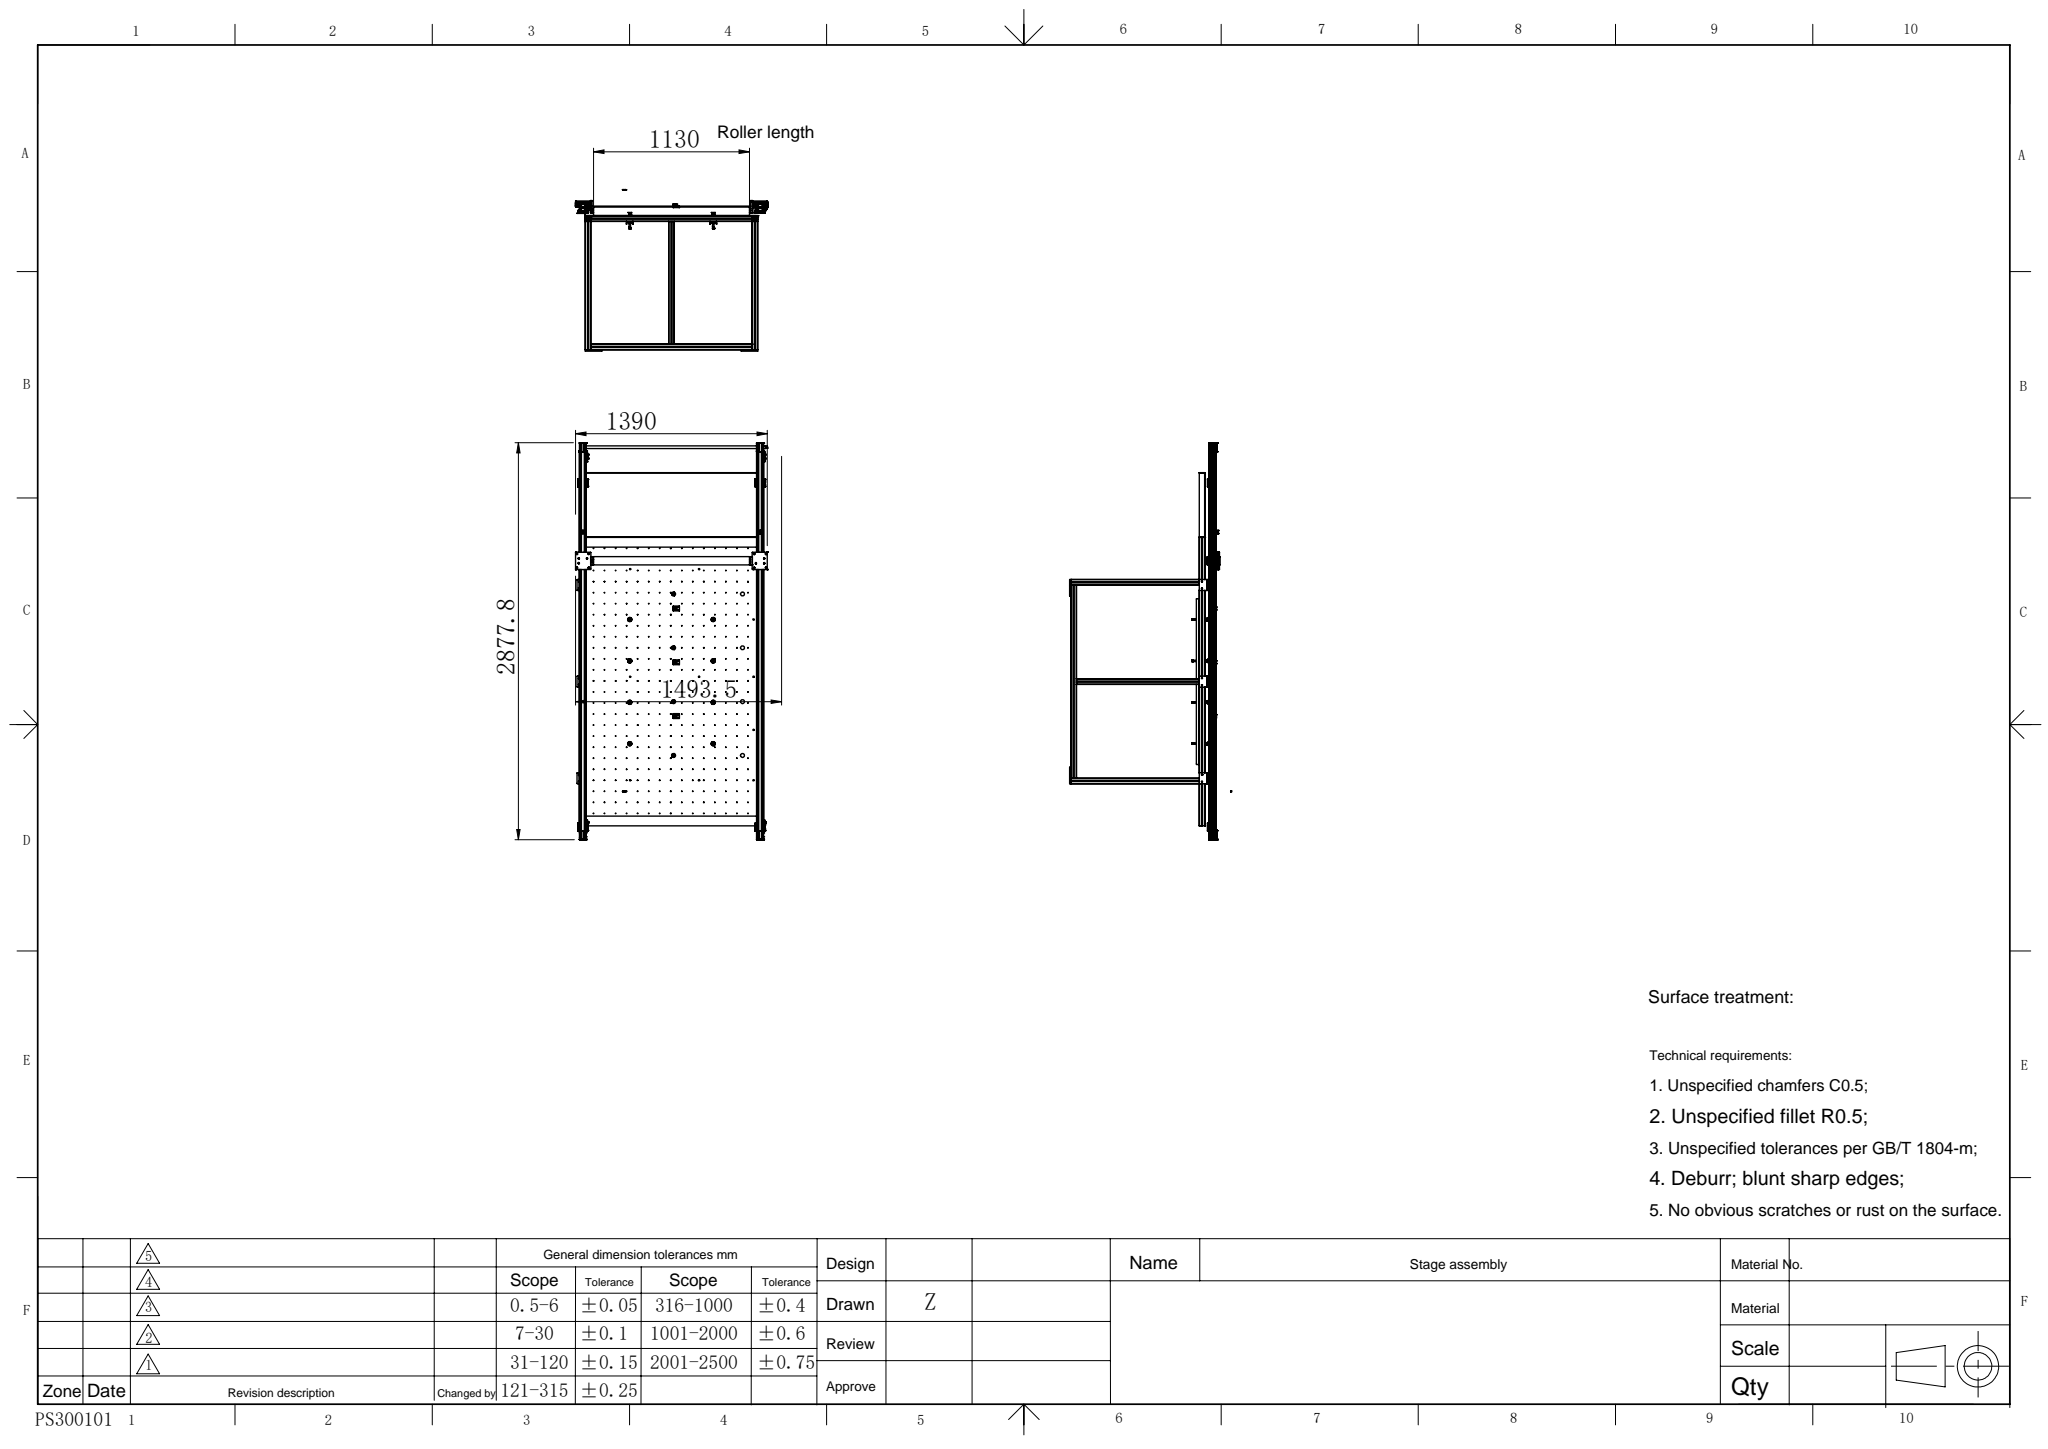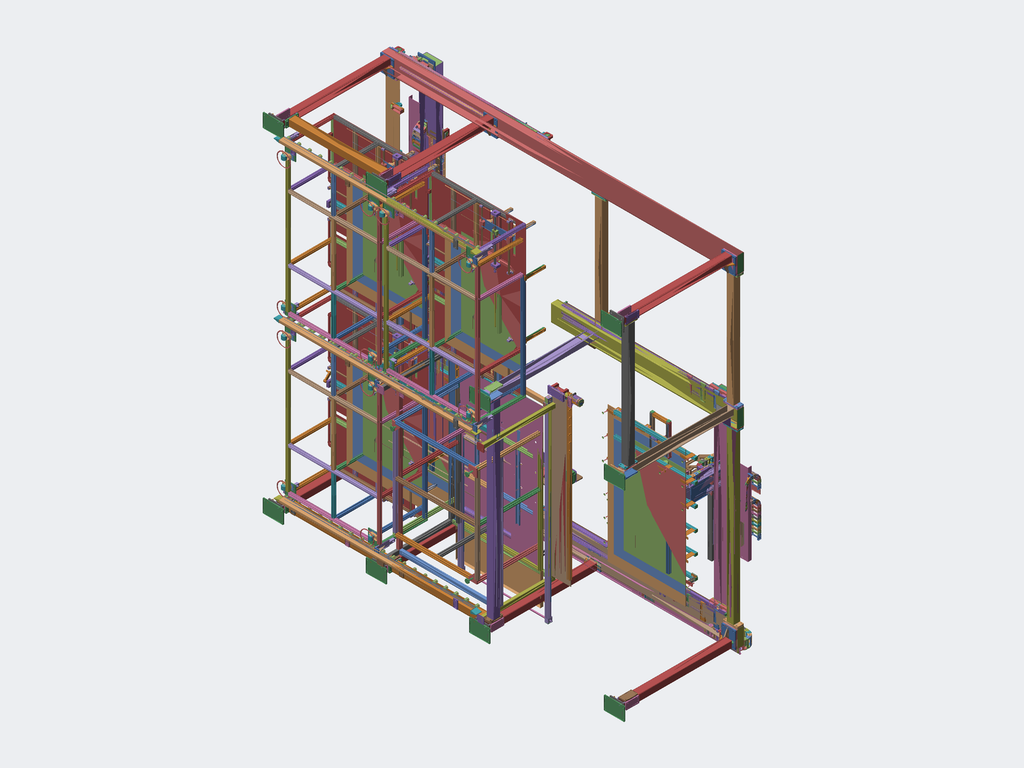Assembly | SolidWorks | 269 different items | 1682 placed
Parts list (item | name | quantity | parent item | size | volume | features):
1 | 57 Stepper and 400W Servo Reducer Pad | x1 | - | - | - | -
2 | (subassembly) | x1 | in 10 | - | - | features ReferencePattern 4, MirrorCompFeat 1
3 | (subassembly) | x1 | in 10 | - | - | features CompositeCurve 1
4 | (subassembly) | x1 | in 10 | - | - | features CompositeCurve 3
5 | (subassembly) | x1 | in 3 | - | - | features CompositeCurve 1, MirrorCompFeat 1, ReferencePattern 1
6 | (subassembly) | x1 | in 4 | - | - | features MirrorCompFeat 1, ReferencePattern 1
7 | (subassembly) | x1 | in 6 | - | 20673869 mm3 | features ReferencePattern 4, CompositeCurve 1, DerivedHolePattern 1
8 | (subassembly) | x1 | in 5 | - | 31071679 mm3 | features ReferencePattern 4, CompositeCurve 1, DerivedHolePattern 1
9 | (subassembly) | x2 | in 7, 8 | 105 x 90.9 x 98 mm | 242700 mm3 | -
10 | (subassembly) | x1 | - | - | - | features ReferencePattern 8, CompositeCurve 2, InContextFeatHolder 2, MirrorCompFeat 2
11 | (subassembly) | x3 | - | - | 40596234 mm3 | features ReferencePattern 157, MirrorCompFeat 6, LocalLPattern 1
12 | (subassembly) | x8 | in 20 | 34 x 24 x 440 mm | 99523 mm3 | -
13 | (subassembly) | x3 | in 3, 10, 15 | 234 x 112 x 120 mm | 1078897 mm3 | -
14 | (subassembly) | x1 | in 10 | 234 x 112 x 120 mm | 1078897 mm3 | -
15 | (subassembly) | x1 | - | - | 35795724 mm3 | features CompositeCurve 8, Belt 1, InContextFeatHolder 1
16 | (subassembly) | x8 | in 21 | 35 x 25 x 45.5 mm | 18401 mm3 | -
17 | (subassembly) | x24 | in 18, 19 | 63.895 x 210.5 x 120 mm | 48532 mm3 | features ReferencePattern 2, DerivedHolePattern 1
18 | (subassembly) | x6 | in 20 | - | 1484218 mm3 | features LocalLPattern 1, ReferencePattern 1
19 | (subassembly) | x6 | in 20 | - | 1567936 mm3 | features ReferencePattern 2, LocalLPattern 1, MirrorCompFeat 1
20 | (subassembly) | x2 | in 7, 8 | - | 15004104 mm3 | features ReferencePattern 15, CompositeCurve 4, MirrorCompFeat 4, LocalLPattern 1
21 | (subassembly) | x1 | in 39 | 2190 x 55.4 x 1350 mm | 56366306 mm3 | features ReferencePattern 7, DerivedHolePattern 1
22 | (subassembly) | x12 | in 18, 19 | 34 x 24 x 680 mm | 167801 mm3 | -
23 | (subassembly) | x2 | - | 2990 x 153 x 120 mm | 4241978 mm3 | features ReferencePattern 36, DerivedHolePattern 1
24 | (subassembly) | x1 | - | 2990 x 153 x 120 mm | 5333989 mm3 | features ReferencePattern 68, LocalLPattern 1
25 | (subassembly) | x1 | in 15 | 30 x 56 x 56 mm | 26536 mm3 | -
26 | (subassembly) | x6 | in 11 | 65 x 310 x 35 mm | 330251 mm3 | -
27 | (subassembly) | x18 | in 36, 37, 38 | 65 x 352 x 35 mm | 373958 mm3 | -
28 | (subassembly) | x3 | in 38 | 62 x 36.8 x 720 mm | 370830 mm3 | -
29 | (subassembly) | x1 | in 15 | 1250 x 163.16 x 142.786 mm | 4866204 mm3 | features CompositeCurve 1
30 | (subassembly) | x2 | in 10 | 250 x 77 x 220 mm | 2116355 mm3 | -
31 | (subassembly) | x1 | in 3 | 250 x 77 x 220 mm | 1248427 mm3 | -
32 | (subassembly) | x2 | in 7, 8 | 30 x 45 x 61.9 mm | 25881 mm3 | -
33 | (subassembly) | x4 | in 10 | 60 x 45 x 2040 mm | 1527513 mm3 | -
34 | (subassembly) | x4 | in 3, 10, 15 | 230 x 112 x 120 mm | 1042878 mm3 | -
35 | (subassembly) | x1 | - | 31 x 72 x 130 mm | 56690 mm3 | -
36 | (subassembly) | x3 | in 11 | 465.166 x 413.18 x 727.5 mm | 2675424 mm3 | -
37 | (subassembly) | x3 | in 11 | 465 x 411 x 721.167 mm | 2675425 mm3 | -
38 | (subassembly) | x3 | in 11 | 866.479 x 413.5 x 727.5 mm | 3012478 mm3 | features MirrorCompFeat 1, ReferencePattern 1
39 | (subassembly) | x1 | - | - | 36230878 mm3 | features ReferencePattern 5, InContextFeatHolder 2, LocalLPattern 1, MirrorCompFeat 1
40 | (subassembly) | x2 | in 7, 8 | 152.95 x 49 x 57.5 mm | 133914 mm3 | features ReferencePattern 5, DerivedHolePattern 1
41 | (subassembly) | x12 | in 18, 19 | 109 x 59.2 x 29.612 mm | 63942 mm3 | features ReferencePattern 7, DerivedHolePattern 1, MirrorCompFeat 1
42 | (subassembly) | x1 | in 39 | - | 15688667 mm3 | features CompositeCurve 1, MirrorCompFeat 1, ReferencePattern 1
43 | (subassembly) | x2 | in 39 | 1200 x 50 x 118 mm | 235695 mm3 | features ReferencePattern 3, LocalLPattern 1
44 | (subassembly) | x3 | in 3 | 60 x 45 x 2850 mm | 1999576 mm3 | -
45 | (subassembly) | x2 | in 46 | - | 2196396 mm3 | features CompositeCurve 3
46 | (subassembly) | x2 | in 42 | - | 6127819 mm3 | features CompositeCurve 10
47 | (subassembly) | x1 | in 4 | 60 x 45 x 920 mm | 875210 mm3 | -
48 | (subassembly) | x2 | in 10 | - | 18345669 mm3 | -
49 | (subassembly) | x8 | in 13, 14, 34 | 89 x 61 x 61 mm | 120828 mm3 | -
50 | (subassembly) | x36 | in 36, 37, 38 | 60 x 55 x 35 mm | 37476 mm3 | -
51 | - | x12 | in 11 | 204.978 x 96 x 204.978 mm | 270055 mm3 | features BaseBody 4, BossThin 1
52 | - | x16 | in 20 | 65 x 34 x 40 mm | 63388 mm3 | features Chamfer 2, HoleWzd 2, Extrusion 1, ICE 1
53 | - | x2 | in 40 | 130 x 30 x 30 mm | 99886 mm3 | features HoleWzd 3, Chamfer 1, Extrusion 1
54 | - | x12 | in 41 | 90 x 30 x 18 mm | 41486 mm3 | features HoleWzd 3, Chamfer 1, Extrusion 1
55 | - | x12 | in 11 | 40 x 30 x 200 mm | 236731 mm3 | features Extrusion 1, HoleWzd 1
56 | - | x26 | in 18, 19, 20 | 40 x 12 x 20 mm | 5424 mm3 | features Chamfer 1, Extrusion 1, HoleWzd 1, ICE 1
57 | - | x4 | in 20 | 46 x 52 x 50 mm | 46820 mm3 | features HoleWzd 2, ICE 2, Chamfer 1, Extrusion 1
58 | - | x4 | in 20 | 430 x 10 x 30 mm | 124086 mm3 | features HoleWzd 2, Chamfer 1, Extrusion 1
59 | - | x2 | in 7, 8 | 230 x 12 x 330 mm | 777440 mm3 | features HoleWzd 3, Chamfer 1, Extrusion 1, Fillet 1, ICE 1
60 | - | x12 | in 18, 19 | 680 x 10 x 47.5 mm | 316323 mm3 | features HoleWzd 2, Chamfer 1, Extrusion 1
61 | - | x2 | in 20 | 380 x 15 x 270 mm | 1473539 mm3 | features ICE 4, HoleWzd 2, Chamfer 1, Extrusion 1
62 | - | x6 | in 11 | 31 x 50 x 50 mm | 48468 mm3 | features BaseBody 1
63 | - | x2 | in 7 | 220 x 12 x 735 mm | 1211217 mm3 | features HoleWzd 8, ICE 2, Chamfer 1, Extrusion 1, Fillet 1
64 | - | x10 | in 7, 8 | 15 x 168 x 15 mm | 28790 mm3 | features Chamfer 1, Extrusion 1, HoleWzd 1, ICE 1, MirrorPattern 1
65 | - | x1 | in 7 | 192 x 15 x 200 mm | 382699 mm3 | features HoleWzd 2, Chamfer 1, Extrusion 1, ICE 1
66 | - | x2 | in 8 | 220 x 12 x 802 mm | 1372017 mm3 | features HoleWzd 8, ICE 2, Chamfer 1, Extrusion 1, Fillet 1
67 | - | x6 | in 11 | 13 x 44.5 x 11 mm | 2225 mm3 | features ICE 3, Chamfer 1, Extrusion 1, RevCut 1
68 | - | x1 | - | 30 x 10 x 126 mm | 36512 mm3 | features HoleWzd 2, Chamfer 1, Extrusion 1
69 | - | x8 | in 16 | 45 x 18.5 x 35 mm | 16639 mm3 | features HoleWzd 2, ICE 2, Chamfer 1, Extrusion 1
70 | - | x4 | - | 60 x 210 x 80 mm | 235958 mm3 | features ICE 3, Chamfer 2, Extrusion 1
71 | - | x3 | in 39 | 60 x 179 x 60 mm | 83421 mm3 | features BaseBody 2
72 | - | x16 | in 13, 14, 34 | 25 x 95 x 100 mm | 157637 mm3 | features HoleWzd 3, ICE 3, Chamfer 2, Extrusion 1
73 | - | x4 | in 13, 14 | 230 x 20 x 100 mm | 414284 mm3 | features HoleWzd 4, Chamfer 1, Extrusion 1, ICE 1
74 | - | x4 | in 13, 14 | 204 x 36 x 36 mm | 132992 mm3 | features ICE 2, Chamfer 1, Revolution 1
75 | - | x16 | in 13, 14, 34 | 18.5 x 40 x 40 mm | 10029 mm3 | features Chamfer 1, Extrusion 1
76 | - | x16 | in 13, 14, 34 | 20 x 25 x 25 mm | 7188 mm3 | features Extrusion 1, HoleWzd 1
77 | - | x4 | in 34 | 169 x 40 x 40 mm | 119602 mm3 | features Chamfer 1, ICE 1, Revolution 1
78 | - | x5 | in 30, 31 | 250 x 77 x 65 mm | 889815 mm3 | features HoleWzd 6, ICE 2, Chamfer 1, Extrusion 1, MirrorPattern 1
79 | - | x6 | in 30, 31 | 70 x 10 x 190 mm | 129097 mm3 | features HoleWzd 2, Chamfer 1, Extrusion 1
80 | - | x2 | in 10 | 20 x 20 x 2135 mm | 670495 mm3 | features Chamfer 1, Extrusion 1
81 | - | x1 | in 10 | 160 x 15 x 160 mm | 370289 mm3 | features HoleWzd 2, Chamfer 1, Extrusion 1
82 | - | x4 | in 3, 10, 15 | 55 x 55 x 57 mm | 102625 mm3 | features BaseBody 1
83 | - | x2 | in 3, 15 | 120 x 117 x 50 mm | 147908 mm3 | features ICE 3, Chamfer 2, HoleWzd 2, Extrusion 1, MirrorSolid 1
84 | - | x4 | in 34 | 230 x 20 x 100 mm | 391656 mm3 | features HoleWzd 3, Chamfer 1, Extrusion 1, ICE 1
85 | - | x3 | in 11 | - | 21852981 mm3 | features WeldCornerFeat 2, 3DProfileFeature 1, WeldMemberFeat 1, WeldmentFeature 1
86 | - | x12 | in 18, 19 | 1200 x 40 x 40 mm | 725812 mm3 | features WeldMemberFeat 1, WeldmentFeature 1
87 | - | x1 | in 39 | 1250 x 970 x 2090 mm | 12416282 mm3 | features ICE 8, Extrusion 1
88 | - | x2 | in 20 | 1940 x 40 x 280 mm | 2830666 mm3 | features WeldMemberFeat 1, WeldmentFeature 1
89 | - | x1 | in 3 | 5030 x 162 x 315 mm | 22440671 mm3 | features ICE 11, HoleWzd 10, Chamfer 1, MirrorSolid 1, WeldMemberFeat 1, WeldmentFeature 1
90 | - | x1 | in 39 | 1590 x 1030 x 1350 mm | 17668090 mm3 | features HoleWzd 4, ICE 3, 3DProfileFeature 1, WeldCornerFeat 1, WeldMemberFeat 1, WeldmentFeature 1
91 | - | x1 | in 10 | 2745 x 1798 x 315 mm | 19263192 mm3 | features ICE 8, HoleWzd 5, MirrorSolid 4, WeldMemberFeat 2, LPattern 1, WeldCornerFeat 1, WeldmentFeature 1
92 | - | x1 | in 4 | 2945 x 142 x 275 mm | 8968186 mm3 | features HoleWzd 7, ICE 5, MirrorSolid 3, Chamfer 2, WeldMemberFeat 1, WeldmentFeature 1
93 | - | x2 | in 10 | - | - | features RefSurface 2
94 | - | x1 | in 10 | 2525 x 210 x 100 mm | 3620734 mm3 | features ICE 3, HoleWzd 2, WeldMemberFeat 2, LPattern 1, MirrorSolid 1, WeldCornerFeat 1, WeldmentFeature 1
95 | - | x1 | in 10 | 4500 x 230 x 153.7 mm | 8314769 mm3 | features ICE 5, HoleWzd 3, MirrorSolid 2, WeldMemberFeat 2, LPattern 1, WeldCornerFeat 1, WeldmentFeature 1
96 | - | x3 | in 23, 24 | 2990 x 95 x 120 mm | 3021491 mm3 | features ICE 5, MirrorSolid 2, HoleWzd 1, WeldMemberFeat 1, WeldmentFeature 1
97 | - | x1 | in 10 | 5240 x 145 x 265 mm | 27147429 mm3 | features ICE 9, HoleWzd 7, DeleteBody 1, MirrorSolid 1, WeldCornerFeat 1, WeldMemberFeat 1, WeldmentFeature 1
98 | - | x1 | in 10 | 5240 x 145 x 265 mm | 23826914 mm3 | features ICE 7, HoleWzd 6, Cut 1, DeleteBody 1, LPattern 1, MirrorSolid 1, WeldCornerFeat 1, WeldMemberFeat 1, WeldmentFeature 1
99 | - | x7 | in 10 | 200 x 1668 x 300 mm | 4715517 mm3 | features ICE 6, HoleWzd 4, CirPattern 2, DeleteBody 1, MirrorSolid 1, RefAxis 1, WeldCornerFeat 1, WeldMemberFeat 1, WeldmentFeature 1
100 | - | x3 | in 10 | 1395 x 100 x 190 mm | 2190418 mm3 | features HoleWzd 1, ICE 1, MirrorSolid 1, WeldMemberFeat 1, WeldmentFeature 1
101 | - | x1 | in 10 | 2825 x 100 x 190 mm | 3924535 mm3 | features HoleWzd 1, ICE 1, MirrorSolid 1, WeldMemberFeat 1, WeldmentFeature 1
102 | - | x1 | in 10 | 1845 x 100 x 190 mm | 2736119 mm3 | features HoleWzd 1, ICE 1, MirrorSolid 1, WeldMemberFeat 1, WeldmentFeature 1
103 | - | x2 | in 10 | 1695 x 100 x 210 mm | 2614218 mm3 | features HoleWzd 1, ICE 1, MirrorSolid 1, WeldMemberFeat 1, WeldmentFeature 1
104 | - | x6 | in 11 | 59 x 25 x 25 mm | 17907 mm3 | features BaseBody 4
105 | - | x1 | in 39 | 2090 x 2.5 x 1250 mm | 5366829 mm3 | features HoleWzd 3, ICE 3, Fillet 2, Extrusion 1
106 | - | x1 | in 15 | 1748 x 110 x 139.4 mm | 4195006 mm3 | features Fillet 2, ICE 2, Extrusion 1
107 | - | x28 | in 17, 20 | 15 x 46 x 15 mm | 3087 mm3 | features BaseBody 1
108 | - | x8 | in 16 | 26 x 10.5 x 26 mm | 1762 mm3 | features BaseBody 2
109 | - | x2 | in 32 | 30 x 45 x 61.9 mm | 24324 mm3 | features BaseBody 3
110 | - | x1 | in 15 | 1374 x 89 x 40 mm | 612800 mm3 | features Extrusion 1, ICE 1, MirrorPattern 1
111 | - | x1 | in 29 | 1200 x 10 x 80 mm | 959446 mm3 | features Extrusion 1, ICE 1
112 | - | x2 | in 15 | 86 x 60.5 x 139.4 mm | 512577 mm3 | features BaseBody 1
113 | - | x2 | in 15 | 45 x 38 x 2380 mm | 3190099 mm3 | features ICE 3, LPattern 2, BaseBody 1, RevCut 1
114 | - | x2 | in 15 | 86 x 25 x 53.5 mm | 94926 mm3 | features ICE 15, Chamfer 1, Extrusion 1, MirrorPattern 1, RevCut 1, Revolution 1
115 | - | x6 | in 3, 10 | 13.6 x 15.5 x 27.7 mm | 2033 mm3 | features BaseBody 1
116 | - | x74 | in 23, 24 | 68 x 13 x 13 mm | 3917 mm3 | features BaseBody 1
117 | - | x1 | in 3 | 80 x 59.15 x 3062 mm | 2509466 mm3 | features BossThin 1, ExtruThin 1
118 | - | x6 | in 30, 31 | 105 x 8 x 57 mm | 39266 mm3 | features HoleWzd 1, WeldMemberFeat 1, WeldmentFeature 1
119 | - | x8 | in 48 | 15.82 x 15.82 x 12 mm | 1643 mm3 | features BaseBody 1
120 | - | x8 | in 48 | 34 x 19.5 x 56.8 mm | 30476 mm3 | features BaseBody 1
121 | - | x2 | in 48 | 20 x 70 x 12 mm | 2355 mm3 | features BaseBody 1
122 | - | x6 | in 48 | 27 x 19 x 20 mm | 1847 mm3 | features BaseBody 1
123 | - | x2 | in 48 | 1.5 x 54 x 30 mm | 1466 mm3 | features BaseBody 1
124 | - | x6 | in 48 | 27.5 x 14 x 16 mm | 2237 mm3 | features BaseBody 1
125 | - | x2 | in 48 | 175 x 66 x 2404 mm | 15856732 mm3 | features BaseBody 3
126 | - | x8 | in 12 | 15 x 12.5 x 440 mm | 69027 mm3 | features ICE 2, BaseBody 1, HoleWzd 1
127 | - | x2 | in 48 | 270 x 54 x 195 mm | 1409975 mm3 | features BaseBody 1
128 | - | x2 | in 48 | 58.084 x 15.975 x 10 mm | 3195 mm3 | features BaseBody 3
129 | - | x4 | in 48 | 32 x 93.5 x 175 mm | 238017 mm3 | features BaseBody 1
130 | - | x4 | in 48 | 8 x 31 x 160 mm | 21339 mm3 | features BaseBody 1
131 | - | x4 | in 48 | 12 x 16 x 130 mm | 19917 mm3 | features BaseBody 1
132 | - | x2 | in 48 | 2454 x 50 x 130 mm | 330700 mm3 | features BaseBody 1
133 | - | x2 | in 48 | 64 x 15 x 7.5 mm | 6074 mm3 | features BaseBody 1
134 | - | x2 | in 48 | 1.5 x 10 x 2344 mm | 35160 mm3 | features BaseBody 1
135 | - | x2 | in 15 | 150 x 16 x 16 mm | 30147 mm3 | features ICE 7, RevCut 2, Chamfer 1, Revolution 1
136 | - | x9 | in 28, 36, 37 | 25 x 25 x 720 mm | 328967 mm3 | features ICE 5, Chamfer 2, Extrusion 1
137 | - | x12 | in 22 | 15 x 12.5 x 680 mm | 106806 mm3 | features ICE 2, BaseBody 1, HoleWzd 1
138 | - | x1 | in 29 | 60 x 60 x 1250 mm | 3405863 mm3 | features ICE 2, Extrusion 1, MirrorPattern 1
139 | - | x1 | in 29 | 1250 x 145.623 x 130.346 mm | 500895 mm3 | features ICE 5, Fillet 2, Extrusion 1, LPattern 1, Sweep 1
140 | - | x2 | in 10 | 80 x 59.15 x 2252 mm | 1851098 mm3 | features BossThin 1, ExtruThin 1
141 | - | x2 | in 15 | 50 x 38.5 x 23.5 mm | 34722 mm3 | features Extrusion 1, ICE 1
142 | - | x12 | in 19 | 20 x 20 x 15 mm | 3713 mm3 | features Extrusion 1, HoleWzd 1
143 | - | x4 | in 3, 10 | 6 x 9 x 250 mm | 7894 mm3 | features Extrusion 1, HoleWzd 1
144 | - | x18 | in 36, 37, 38 | 20 x 20 x 690 mm | 216754 mm3 | features Chamfer 1, Extrusion 1
145 | - | x1 | in 15 | 1794 x 1094 x 2450 mm | 14966587 mm3 | features ICE 8, Extrusion 1
146 | - | x1 | in 42 | 92 x 60 x 12 mm | 51329 mm3 | features MirrorStock 1
147 | - | x1 | in 39 | 1250 x 470 x 42 mm | 1441666 mm3 | features EdgeFlange 1, FlatPattern 1, ICE 1, LPattern 1, SMBaseFlange 1, SheetMetal 1
148 | - | x32 | in 12, 22 | 34 x 19.5 x 57.8 mm | 30496 mm3 | features BaseBody 1
149 | - | x6 | in 39 | 80 x 60 x 60 mm | 27475 mm3 | features HoleWzd 2, EdgeFlange 1, Fillet 1, FlatPattern 1, SMBaseFlange 1, SheetMetal 1
150 | - | x2 | in 43 | 1200 x 50 x 20 mm | 201265 mm3 | features EdgeFlange 1, Fillet 1, FlatPattern 1, HoleWzd 1, ICE 1, SMBaseFlange 1, SheetMetal 1
151 | - | x2 | in 42 | 126 x 110 x 10 mm | 134120 mm3 | features HoleWzd 2, Chamfer 1, Extrusion 1
152 | - | x1 | in 42 | 92 x 60 x 12 mm | 51329 mm3 | features HoleWzd 2, ICE 2, Chamfer 1, Extrusion 1, Fillet 1
153 | - | x1 | in 42 | 60 x 60 x 1176 mm | 3172741 mm3 | features HoleWzd 2, ICE 2, Extrusion 1
154 | - | x1 | in 42 | 20 x 20 x 1300 mm | 408407 mm3 | features Extrusion 1
155 | - | x2 | in 46 | 39 x 39 x 49 mm | 38785 mm3 | features ICE 15, RevCut 7, CirPattern 3, Emboss 2, MirrorPattern 1, Revolution 1
156 | - | x2 | in 45 | 105 x 79 x 220 mm | 575496 mm3 | features BaseBody 33
157 | - | x6 | in 46 | 79.5 x 156 x 47 mm | 158160 mm3 | features BaseBody 3, MoveFace 2, ICE 1
158 | - | x2 | in 46 | 79.5 x 156 x 47 mm | 157908 mm3 | features BaseBody 3, MoveFace 2, ICE 1
159 | - | x32 | in 18, 19, 20 | 40 x 5 x 40 mm | 7913 mm3 | features Extrusion 1, Fillet 1
160 | - | x58 | in 17, 18, 19, 20, 43 | 28 x 118 x 28 mm | 8607 mm3 | features BaseBody 3
161 | - | x2 | in 46 | 87.3 x 177.09 x 47 mm | 222121 mm3 | features MoveFace 4, BaseBody 3, ICE 2
162 | - | x2 | in 46 | 87.3 x 177.09 x 47 mm | 215586 mm3 | features BaseBody 3, MoveFace 3, ICE 2
163 | - | x4 | in 46 | 105 x 52 x 165 mm | 515156 mm3 | features BaseBody 3
164 | - | x2 | in 46 | 105 x 52 x 220 mm | 691685 mm3 | features BaseBody 3
165 | - | x2 | in 46 | 105 x 52 x 126 mm | 392725 mm3 | features BaseBody 4
166 | - | x4 | in 46 | 60 x 60 x 112 mm | 219786 mm3 | features BaseBody 3
167 | - | x4 | in 46 | - | - | features RefSurface 50
168 | - | x2 | in 46 | 35 x 44 x 44 mm | 38152 mm3 | features BaseBody 10
169 | - | x2 | in 46 | - | - | features RefSurface 12
170 | - | x8 | in 46 | 59.5 x 59.5 x 14.7 mm | 28959 mm3 | features HoleWzd 3, ICE 3, CirPattern 2, Fillet 2, Chamfer 1, Cut 1, Extrusion 1, MirrorPattern 1
171 | - | x1 | in 7 | 135 x 141 x 169.1 mm | 931698 mm3 | features BaseBody 2
172 | - | x2 | in 46 | 106 x 62 x 74 mm | 204451 mm3 | features BaseBody 13, ICE 5, Chamfer 3
173 | - | x2 | in 46 | 86 x 62 x 74 mm | 199634 mm3 | features BaseBody 13, ICE 6, Chamfer 3
174 | - | x4 | in 46 | 59.5 x 62 x 74 mm | 191803 mm3 | features BaseBody 13, ICE 4, Chamfer 2
175 | - | x2 | in 46 | 79.5 x 62 x 74 mm | 200359 mm3 | features BaseBody 13, ICE 3, Chamfer 2
176 | - | x2 | in 46 | 106 x 62 x 74 mm | 204451 mm3 | features BaseBody 13, ICE 5, Chamfer 3, DeleteBody 1, MirrorSolid 1
177 | - | x2 | in 46 | 86 x 62 x 74 mm | 199635 mm3 | features BaseBody 13, ICE 6, Chamfer 3, DeleteBody 1, MirrorSolid 1
178 | - | x2 | in 46 | 59.5 x 62 x 74 mm | 191804 mm3 | features BaseBody 13, ICE 4, Chamfer 2, DeleteBody 1, MirrorSolid 1
179 | - | x2 | in 46 | 79.5 x 62 x 74 mm | 200359 mm3 | features BaseBody 13, ICE 3, Chamfer 2, DeleteBody 1, MirrorSolid 1
180 | - | x4 | in 46 | 60.5 x 118.5 x 60.5 mm | 241824 mm3 | features MBimport 1
181 | - | x4 | in 46 | - | - | features RefSurface 11
182 | - | x1 | in 35 | 31 x 72 x 130 mm | 55783 mm3 | features BaseBody 1
183 | - | x16 | in 33, 44, 47 | 60 x 39.001 x 97.7 mm | 170718 mm3 | features BaseBody 1
184 | - | x1 | in 47 | 28 x 26 x 920 mm | 533776 mm3 | features ICE 2, BaseBody 1, HoleWzd 1
185 | - | x3 | in 44 | 28 x 26 x 2850 mm | 1658147 mm3 | features ICE 2, BaseBody 1, HoleWzd 1
186 | - | x4 | in 33 | 28 x 26 x 2040 mm | 1186082 mm3 | features BaseBody 1, HoleWzd 1, ICE 1
187 | - | x1 | in 10 | 40.704 x 156.673 x 40.704 mm | 14106 mm3 | features BaseBody 2
188 | - | x1 | in 10 | 224 x 110 x 250 mm | 1662624 mm3 | features BaseBody 14
189 | - | x9 | in 28, 36, 37 | 36.8 x 62 x 50 mm | 41876 mm3 | features BaseBody 1
190 | - | x3 | in 39 | 120 x 120 x 10 mm | 110461 mm3 | features Extrusion 1, HoleWzd 1
191 | - | x18 | in 36, 37, 38 | 54 x 41 x 96 mm | 148221 mm3 | features BaseBody 1
192 | - | x4 | in 3, 4, 10, 15 | - | - | features RefSurface 26, BaseBody 15
193 | - | x2 | in 5, 6 | - | - | features RefSurface 26, BaseBody 20
194 | - | x1 | in 7 | - | - | features RefSurface 65
195 | - | x1 | in 10 | 110 x 224 x 250 mm | 2228860 mm3 | features BaseBody 34
196 | - | x1 | in 7 | - | - | features BaseBody 60, RefSurface 7
197 | - | x10 | in 3, 10, 31 | 13 x 15.011 x 68 mm | 5094 mm3 | features BaseBody 1
198 | - | x10 | in 3, 10, 31 | 12 x 18 x 38 mm | 5849 mm3 | features BaseBody 1
199 | - | x2 | in 40 | 39.583 x 28.95 x 18 mm | 7377 mm3 | features BaseBody 1
200 | - | x2 | in 32 | 24.119 x 17 x 10.238 mm | 1557 mm3 | features BaseBody 1
201 | - | x6 | in 11, 20, 21 | 2010 x 50 x 1150 mm | 11975475 mm3 | features ICE 5, Extrusion 1
202 | - | x120 | in 17, 41 | 28.619 x 17.5 x 12.5 mm | 2253 mm3 | features BaseBody 1
203 | - | x24 | in 40, 41 | 33.351 x 25 x 15 mm | 4442 mm3 | features BaseBody 1
204 | - | x2 | in 5, 6 | 384.7 x 122 x 879.7 mm | 13861724 mm3 | features BaseBody 11
205 | - | x1 | in 4 | 1047 x 122 x 230 mm | 15190033 mm3 | features BaseBody 6, LPattern 1
206 | - | x16 | in 49 | 61 x 61 x 2.5 mm | 4721 mm3 | features ICE 2, BaseBody 1
207 | - | x8 | in 49 | 84 x 54.65 x 54.249 mm | 111386 mm3 | features CirPattern 1, Cut 1, HoleWzd 1, ICE 1, WeldMemberFeat 1, WeldmentFeature 1
208 | - | x36 | in 50 | 60 x 51 x 20 mm | 29381 mm3 | features BaseBody 1
209 | - | x8 | in 19, 20 | 94 x 36 x 36 mm | 78823 mm3 | features BaseBody 2
210 | - | x1 | in 5 | 13 x 13 x 17.5 mm | 922.307 mm3 | features BaseBody 1
211 | - | x1 | in 3 | 90 x 90.211 x 179.85 mm | 785388 mm3 | features BaseBody 7
212 | - | x1 | in 3 | 90.02 x 90.185 x 188 mm | 989855 mm3 | features BaseBody 2
213 | - | x6 | in 10 | 127 x 65 x 37 mm | 109868 mm3 | features BaseBody 1
214 | - | x1 | in 4 | - | 2054187 mm3 | features BaseBody 18, LPattern 4
215 | - | x3 | in 2, 3 | - | - | features BaseBody 38, LPattern 5
216 | - | x2 | in 5, 6 | - | 1173984 mm3 | features BaseBody 14, LPattern 4
217 | - | x6 | in 11 | 630 x 56 x 28 mm | 285971 mm3 | features BaseBody 1
218 | - | x3 | in 11 | 2220 x 2 x 1390 mm | 5915480 mm3 | features Fillet 2, ICE 2, FlatPattern 1, HoleWzd 1, SMBaseFlange 1, SheetMetal 1
219 | - | x2 | in 5, 6 | 102 x 570 x 30 mm | 144671 mm3 | features HoleWzd 3, Fillet 1, FlatPattern 1, SMBaseFlange 1, SheetMetal 1
220 | - | x2 | in 6, 8 | 115 x 30 x 60 mm | 24246 mm3 | features HoleWzd 3, Fillet 1, FlatPattern 1, SMBaseFlange 1, SheetMetal 1
221 | - | x1 | in 3 | 202 x 70 x 3780 mm | 2020331 mm3 | features HoleWzd 3, Fillet 1, FlatPattern 1, ICE 1, SMBaseFlange 1, SheetMetal 1
222 | - | x2 | in 5, 6 | 225 x 23 x 70 mm | 48684 mm3 | features HoleWzd 3, Fillet 1, FlatPattern 1, ICE 1, Jog 1, SMBaseFlange 1, SheetMetal 1
223 | - | x18 | in 36, 37, 38 | 12 x 42 x 42 mm | 10328 mm3 | features BaseBody 1
224 | - | x2 | in 2 | 151 x 23 x 2540 mm | 1429422 mm3 | features HoleWzd 3, Fillet 1, FlatPattern 1, SMBaseFlange 1, SheetMetal 1
225 | - | x5 | in 2 | 145 x 53 x 145 mm | 95976 mm3 | features FlatPattern 3, HoleWzd 2, SMBaseFlange 2, SheetMetal 2, Fillet 1, MirrorSolid 1
226 | - | x2 | in 3, 4 | 339 x 20 x 110 mm | 86427 mm3 | features HoleWzd 3, EdgeFlange 1, Fillet 1, FlatPattern 1, ICE 1, SMBaseFlange 1, SheetMetal 1
227 | - | x6 | in 3, 10 | 25 x 25 x 1.5 mm | 877.913 mm3 | features HoleWzd 2, Fillet 1, FlatPattern 1, SMBaseFlange 1, SheetMetal 1
228 | - | x1 | in 5 | 40 x 25 x 25 mm | 1391 mm3 | features Fillet 2, FlatPattern 1, HoleWzd 1, ICE 1, SMBaseFlange 1, SheetMetal 1
229 | - | x1 | in 4 | 162 x 40 x 950 mm | 374388 mm3 | features HoleWzd 3, Fillet 1, FlatPattern 1, SMBaseFlange 1, SheetMetal 1
230 | - | x1 | in 4 | 202 x 70 x 1205 mm | 643774 mm3 | features HoleWzd 3, Fillet 1, FlatPattern 1, ICE 1, SMBaseFlange 1, SheetMetal 1
231 | - | x1 | in 10 | 36.2 x 72.7 x 25 mm | 3370 mm3 | features Fillet 2, FlatPattern 1, HoleWzd 1, ICE 1, SMBaseFlange 1, SheetMetal 1
232 | - | x48 | in 17, 18, 19 | 35 x 139 x 120 mm | 34584 mm3 | features ICE 5, Fillet 2, ExtruThin 1, FlatPattern 1, FlattenBends 1, ProcessBends 1, SheetMetal 1
233 | - | x6 | in 19 | 53 x 80 x 70 mm | 26067 mm3 | features ICE 11, Fillet 2, ExtruThin 1, FlatPattern 1, FlattenBends 1, ProcessBends 1, SheetMetal 1
234 | - | x16 | in 13, 14, 34 | 16 x 62 x 62 mm | 30543 mm3 | features BaseBody 1
235 | - | x36 | in 50 | 60 x 35 x 4 mm | 8095 mm3 | features Extrusion 1, Fillet 1
236 | - | x1 | in 10 | 40 x 127 x 2 mm | 8841 mm3 | features ICE 2, Extrusion 1, Fillet 1
237 | - | x2 | in 20 | 50 x 78.5 x 48.5 mm | 6398 mm3 | features ICE 2, Extrusion 1, Fillet 1, FlatPattern 1, SheetMetal 1, SolidToSheetMetal 1
238 | - | x1 | in 7 | 200 x 84 x 50 mm | 47784 mm3 | features ICE 2, Extrusion 1
239 | - | x1 | in 10 | 40 x 162 x 2 mm | 11517 mm3 | features ICE 2, Extrusion 1, Fillet 1
240 | - | x6 | in 19 | 110 x 44 x 3 mm | 13820 mm3 | features Fillet 2, Cut 1, Extrusion 1, ICE 1
241 | - | x2 | in 20 | 130 x 40 x 3 mm | 14438 mm3 | features Extrusion 1, Fillet 1, ICE 1
242 | - | x2 | in 20 | 80 x 80 x 12 mm | 37889 mm3 | features ICE 5, Fillet 3, Extrusion 1, LPattern 1
243 | - | x2 | in 5, 6 | 350 x 140 x 101.5 mm | 86053 mm3 | features ICE 3, BossThin 1, Extrusion 1, Fillet 1
244 | - | x1 | in 5 | 440 x 100 x 50 mm | 150958 mm3 | features ICE 4, Extrusion 1, Fillet 1, FlatPattern 1, Rip 1, SheetMetal 1, Shell 1, SolidToSheetMetal 1
245 | - | x3 | in 11 | 32 x 6 x 6 mm | 521.254 mm3 | features BaseBody 1
246 | - | x1 | in 3 | 120 x 40 x 1500 mm | 161482 mm3 | features ICE 4, ExtruThin 1, Fillet 1, FlatPattern 1, FlattenBends 1, ProcessBends 1, SheetMetal 1
247 | - | x1 | in 4 | 120 x 40 x 1200 mm | 129437 mm3 | features ICE 4, ExtruThin 1, Fillet 1, FlatPattern 1, FlattenBends 1, ProcessBends 1, SheetMetal 1
248 | - | x2 | in 20 | 2 x 45 x 65 mm | 5159 mm3 | features Fillet 1, FlatPattern 1, HoleWzd 1, ICE 1, SMBaseFlange 1, SheetMetal 1
249 | - | x1 | in 35 | 22 x 3 x 22 mm | 907.041 mm3 | features FlatPattern 1, HoleWzd 1, SMBaseFlange 1, SheetMetal 1
250 | - | x12 | in 11 | 160 x 8 x 190 mm | 239568 mm3 | features HoleWzd 3, Chamfer 1, Extrusion 1
251 | - | x18 | in 36, 37, 38 | 80 x 30 x 65 mm | 99631 mm3 | features ICE 5, HoleWzd 4, Chamfer 1, Extrusion 1
252 | - | x6 | in 36, 37 | 465 x 8 x 105 mm | 386163 mm3 | features HoleWzd 3, Chamfer 1, Extrusion 1
253 | - | x9 | in 36, 37, 38 | 62 x 45 x 45 mm | 70731 mm3 | features HoleWzd 2, Chamfer 1, Extrusion 1, ICE 1, MirrorPattern 1
254 | - | x18 | in 27 | 65 x 352 x 20 mm | 218982 mm3 | features HoleWzd 3, Chamfer 1, Extrusion 1, Fillet 1, LPattern 1
255 | - | x6 | in 26 | 65 x 310 x 20 mm | 194175 mm3 | features HoleWzd 3, Chamfer 1, Extrusion 1, Fillet 1
256 | - | x74 | in 23, 24 | 40 x 40 x 50 mm | 60319 mm3 | features Extrusion 1
257 | - | x3 | in 38 | 865 x 8 x 105 mm | 723256 mm3 | features HoleWzd 3, Chamfer 1, Extrusion 1
258 | - | x3 | in 11 | 14 x 715 x 14 mm | 108794 mm3 | features Chamfer 1, Extrusion 1, ICE 1
259 | - | x1 | in 21 | 2190 x 15 x 1350 mm | 44243626 mm3 | features HoleWzd 3, Chamfer 1, Extrusion 1, PLine 1
260 | - | x18 | in 27 | 30 x 352 x 15 mm | 154976 mm3 | features Extrusion 1, Fillet 1, HoleWzd 1
261 | - | x6 | in 26 | 30 x 310 x 15 mm | 136076 mm3 | features Extrusion 1, Fillet 1, HoleWzd 1
262 | - | x2 | in 5, 6 | 230 x 12 x 670 mm | 1812577 mm3 | features HoleWzd 6, Chamfer 1, Extrusion 1, MirrorPattern 1
263 | - | x2 | in 5, 6 | 250 x 12 x 306 mm | 899864 mm3 | features HoleWzd 5, Chamfer 2, Extrusion 1, ICE 1
264 | - | x4 | in 5, 6 | 291 x 12 x 134 mm | 221726 mm3 | features HoleWzd 2, Extrusion 1, ICE 1
265 | - | x9 | in 10 | 300 x 80 x 200 mm | 745614 mm3 | features Chamfer 2, HoleWzd 2, Extrusion 1, ICE 1, SketchPattern 1
266 | - | x8 | in 20 | 60 x 10 x 40 mm | 21259 mm3 | features HoleWzd 2, Chamfer 1, Extrusion 1
267 | - | x4 | in 9 | 71.5 x 90.9 x 38 mm | 121350 mm3 | features BaseBody 1
268 | P50DJZ-750W Motor Mount-750W-02 | x1 | - | - | - | -
269 | Inovance Servo Motor MS1H1-40B30CB-A331Z-02 | x1 | - | - | - | -
Mates (type | each side: item.copy, entity, surface, feature), first 226 of 1083 lines:
In the top assembly
Width | 85.1 face plane Aluminium Profile 40 X 40W X R4.5(1) | 85.1 face plane Aluminium Profile 40 X 40W X R4.5(1) | assembly face | assembly face
Coincident | assembly face | assembly face | 2 times
DistanceDim | assembly face | 85.1 face plane Aluminium Profile 40 X 40W X R4.5(1)
Coincident | 85.1 face plane Aluminium Profile 40 X 40W X R4.5(1) | 85.2 face plane Aluminium Profile 40 X 40W X R4.5(1)
DistanceDim | 85.2 face plane Aluminium Profile 40 X 40W X R4.5(1) | 85.1 face plane Aluminium Profile 40 X 40W X R4.5(1)
Coincident | assembly face | 51.1 face plane Extrude-Thin Wall 1
Coincident | 51.1 face plane Extrude-Thin Wall 1 | 51.2 face plane Extrude-Thin Wall 1
DistanceDim | 85.1 face plane Aluminium Profile 40 X 40W X R4.5(1) | assembly face
DistanceDim | assembly face | assembly face | 2 times
Coincident | 250.1 face plane Boss-Extrude 1 | 96.1 face plane Boss-Extrude 1
Coincident | 96.1 face plane Boss-Extrude 2 | 96.2 face plane Boss-Extrude 2
Coincident | 96.1 face plane Boss-Extrude 1 | 96.2 face plane Mirror 1
Coincident | 96.1 face plane Boss-Extrude 1 | 96.3 face plane Boss-Extrude 1
Coincident | 96.1 face plane Boss-Extrude 2 | 96.3 face plane Boss-Extrude 2
DistanceDim | 90.1 face plane Square Tube 60 X 60 X 3.2(1) | 99.1 face plane Square Tube 100 X 100 X 4.0(2) | 2 times
Coincident | 265.1 face plane Boss-Extrude 1 | assembly face | 2 times
Coincident | 265.2 face plane Boss-Extrude 1 | 96.1 face plane Boss-Extrude 2
DistanceDim | 96.1 face plane Boss-Extrude 1 | 99.2 face plane Square Tube 100 X 100 X 4.0(2)
Width | 96.1 face plane Rectangular Tube 80X40X3(1) | 96.2 face plane Rectangular Tube 80X40X3(1) | 99.3 face plane Square Tube 100 X 100 X 4.0(2) | 99.2 face plane Square Tube 100 X 100 X 4.0(2)
DistanceDim | 96.1 face plane Rectangular Tube 80X40X3(1) | 100.1 face plane Square Tube 100 X 100 X 3.2(1)
Coincident | 85.2 face plane Aluminium Profile 40 X 40W X R4.5(1) | 96.1 face plane Boss-Extrude 1
Coincident | 51.2 face plane Extrude-Thin Wall 1 | 96.1 face plane Boss-Extrude 2
Width | assembly face | assembly face | 100.2 face plane Square Tube 100 X 100 X 3.2(1) | 100.1 face plane Square Tube 100 X 100 X 3.2(1)
Coincident | 55.1 face plane Boss-Extrude 1 | 70.1 face plane Boss-Extrude 2 | 2 times
Coincident | 96.1 face plane Boss-Extrude 2 | 70.1 face plane Boss-Extrude 1
Coincident | 70.1 face plane Boss-Extrude 2 | 70.2 face plane Boss-Extrude 2
Coincident | 70.1 face plane Boss-Extrude 1 | 70.2 face plane Boss-Extrude 1
Coincident | 55.2 face plane Boss-Extrude 1 | 70.2 face plane Boss-Extrude 2
Coincident | 96.3 face plane Boss-Extrude 2 | 70.3 face plane Boss-Extrude 1
Coincident | 55.3 face plane Boss-Extrude 1 | 70.3 face plane Boss-Extrude 2 | 2 times
Coincident | assembly face | 70.4 face plane Boss-Extrude 1
Coincident | 55.4 face plane Boss-Extrude 1 | 70.4 face plane Boss-Extrude 2 | 2 times
Concentric | 251.1 face | assembly face
Coincident | 136.1 face | assembly face
Parallel | 136.1 face | assembly face
Coincident | 96.2 face plane Boss-Extrude 2 | 70.4 face plane Boss-Extrude 1
Width | 96.3 face plane Rectangular Tube 80X40X3(1) | 96.3 face plane Rectangular Tube 80X40X3(1) | 96.1 face plane Rectangular Tube 80X40X3(1) | 96.2 face plane Rectangular Tube 80X40X3(1)
Coincident | 265.1 face plane Boss-Extrude 1 | 145.1 face plane Boss-Extrude 2
Parallel | 91.1 face plane Square Tube 100 X 100 X 4.0(2) | 145.1 face plane Boss-Extrude 1
Width | 145.1 face plane Boss-Extrude 1 | 145.1 face plane Boss-Extrude 1 | 87.1 face plane Boss-Extrude 3 | 87.1 face plane Boss-Extrude 3
Width | 145.1 face plane Boss-Extrude 1 | 145.1 face plane Boss-Extrude 1 | 87.1 face plane Boss-Extrude 2 | 87.1 face plane Boss-Extrude 2
In subassembly 11
Coincident | 85.3 face plane Aluminium Profile 40 X 40W X R4.5(1) | 250.2 face plane Boss-Extrude 1 | 3 times
Coincident | 85.3 face plane Aluminium Profile 40 X 40W X R4.5(1) | 218.1 face plane Base-Flange 1
Width | 218.1 face plane Base-Flange 1 | 218.1 face plane Base-Flange 1 | 85.3 face plane Aluminium Profile 40 X 40W X R4.5(1) | 85.3 face plane Aluminium Profile 40 X 40W X R4.5(1) | 2 times
Coincident | 85.3 face plane Aluminium Profile 40 X 40W X R4.5(1) | 251.2 face plane Boss-Extrude 1
Width | 251.2 face plane Boss-Extrude 1 | 251.2 face plane Boss-Extrude 1 | 85.3 face plane Aluminium Profile 40 X 40W X R4.5(1) | 85.3 face plane Aluminium Profile 40 X 40W X R4.5(1)
Coincident | 85.3 plane | 251.2 plane
Coincident | 85.3 face plane Aluminium Profile 40 X 40W X R4.5(1) | 251.3 face plane Boss-Extrude 1
Width | 251.3 face plane Boss-Extrude 1 | 251.3 face plane Boss-Extrude 1 | 85.3 face plane Aluminium Profile 40 X 40W X R4.5(1) | 85.3 face plane Aluminium Profile 40 X 40W X R4.5(1)
Parallel | 85.3 face plane Aluminium Profile 40 X 40W X R4.5(1) | 251.3 face plane Boss-Extrude 1
Width | 260.1 face plane Boss-Extrude 1 | 260.2 face plane Boss-Extrude 1 | 218.1 face plane Cut-Extrude 1 | 218.1 face plane Cut-Extrude 1
Coincident | 85.3 face plane Aluminium Profile 40 X 40W X R4.5(1) | 251.4 face plane Boss-Extrude 1 | 2 times
Coincident | 85.3 face plane Aluminium Profile 40 X 40W X R4.5(1) | 255.1 face plane Boss-Extrude 1
Width | 255.1 face plane Boss-Extrude 1 | 255.1 face plane Boss-Extrude 1 | 218.1 face plane Cut-Extrude 2 | 218.1 face plane Cut-Extrude 2
Width | 85.3 face plane Aluminium Profile 40 X 40W X R4.5(1) | 85.3 face plane Aluminium Profile 40 X 40W X R4.5(1) | 255.1 face cylinder Ø9.0 (9) DiameterHole 1
Coincident | 218.1 face plane Base-Flange 1 | 201.1 face plane Boss-Extrude 1
Coincident | 85.3 plane | 201.1 plane
Coincident | 85.3 face plane Aluminium Profile 40 X 40W X R4.5(1) | 217.1 face plane Import 1
Width | 85.3 face plane Aluminium Profile 40 X 40W X R4.5(1) | 218.1 face plane Base-Flange 1 | 217.1 face plane Import 1 | 217.1 face plane Import 1
DistanceDim | 217.1 face plane Import 1 | 217.2 face plane Import 1
Concentric | 136.2 face cylinder Boss-Extrude 4 | 104.1 face cylinder HI_14-25-001                                                                                                                14-1-solid1
Coincident | 136.2 face plane Boss-Extrude 4 | 104.1 face plane HI_14-25-001                                                                                                                14-1-solid1
Concentric | 136.2 face cylinder Cut-Extrude 1 | 104.1 face cylinder HI_14-25-001                                                                                                                14-1-solid1
Concentric | 136.3 face cylinder Cut-Extrude 1 | 104.2 face cylinder HI_14-25-001                                                                                                                14-2-solid1
Concentric | 136.3 face cylinder Boss-Extrude 4 | 104.2 face cylinder HI_14-25-001                                                                                                                14-2-solid1
Concentric | 104.2 face cylinder HI_14-25-001                                                                                                                14-1-solid1 | 258.1 face cylinder Boss-Extrude 1
Coincident | 104.2 face plane HI_14-25-001                                                                                                                14-1-solid1 | 258.1 face plane Boss-Extrude 1
Coincident | 250.2 face plane Boss-Extrude 1 | 51.3 face plane CGL00-D63-001-1-solid1
Slot | 51.3 face cylinder CGL00-D63-001-1-solid1 | 250.2 face cylinder M8 Tapped Hole 2
Slot | 250.2 face cylinder M8 Tapped Hole 2 | 51.3 face cylinder CGL00-D63-001-1-solid1
Coincident | 85.3 face plane Aluminium Profile 40 X 40W X R4.5(1) | 55.5 face plane Boss-Extrude 1
Width | 55.5 face plane Boss-Extrude 1 | 55.5 face plane Boss-Extrude 1 | 85.3 face plane Aluminium Profile 40 X 40W X R4.5(1) | 85.3 face plane Aluminium Profile 40 X 40W X R4.5(1)
Coincident | 261.1 face plane Boss-Extrude 1 | 201.1 face plane Boss-Extrude 1
Coincident | 250.2 face plane Boss-Extrude 1 | 55.5 face plane Boss-Extrude 1
Concentric | 136.2 face cylinder Cut-Extrude 1 | 245.1 face cylinder Import 1
Width | 245.1 face plane Import 1 | 245.1 face plane Import 1 | 136.2 face cylinder Boss-Extrude 4
Concentric | 62.1 face cylinder Import 1 | 67.1 face cylinder Boss-Extrude 1
Coincident | 62.1 face plane Import 1 | 67.1 face plane Boss-Extrude 3
Coincident | 250.3 face plane Boss-Extrude 1 | 67.1 face plane Boss-Extrude 1
Concentric | 250.3 face | 67.1 face cylinder Boss-Extrude 2
In subassembly 26
Coincident | 255.2 face plane Boss-Extrude 1 | 261.2 face plane Boss-Extrude 1 | 3 times
In subassembly 36
Coincident | 251.5 plane | 36.1 plane | 3 times
Concentric | 251.5 face | 144.1 face cylinder Boss-Extrude 1
Coincident | 251.5 face plane Boss-Extrude 1 | 144.1 face plane Boss-Extrude 1
Concentric | 251.5 face | 144.2 face cylinder Boss-Extrude 1
Coincident | 251.5 face plane Boss-Extrude 1 | 144.2 face plane Boss-Extrude 1
Coincident | 251.6 face plane Boss-Extrude 1 | 144.1 face plane Boss-Extrude 1
Concentric | 251.6 face | 144.2 face cylinder Boss-Extrude 1
Concentric | 251.6 face | 144.1 face cylinder Boss-Extrude 1
Concentric | 251.5 face cylinder Cut-Extrude 3 | 223.1 face cylinder Import 1
Coincident | 251.5 face plane Cut-Extrude 3 | 223.1 face plane Import 1
Concentric | 251.6 face cylinder Cut-Extrude 3 | 223.2 face cylinder Import 1
Coincident | 251.6 face plane Cut-Extrude 3 | 223.2 face plane Import 1
Coincident | 223.2 face plane Import 1 | 136.4 face plane Boss-Extrude 1
Concentric | 223.2 face cylinder Import 1 | 136.4 face cylinder Boss-Extrude 1
Concentric | 136.4 face cylinder Boss-Extrude 1 | 189.1 face cylinder Import 1
Parallel | 252.1 face plane Boss-Extrude 1 | 189.1 edge
LimitDistanceDim | 251.6 face plane Boss-Extrude 1 | 252.1 face plane Boss-Extrude 1
Coincident | 252.1 face plane Boss-Extrude 1 | 254.1 face plane Boss-Extrude 1
Concentric | 189.1 face cylinder Import 1 | 253.1 face cylinder Cut-Extrude 1
Coincident | 189.1 face plane Import 1 | 253.1 face plane Boss-Extrude 1
Coincident | 252.1 face plane Boss-Extrude 1 | 253.1 face plane Boss-Extrude 1
Concentric | 252.1 face | 253.1 face cylinder M6 Tapped Hole 1
Concentric | 144.2 face cylinder Boss-Extrude 1 | 191.1 face cylinder Import 1
Coincident | 252.1 face plane Boss-Extrude 1 | 191.1 face plane Import 1
Concentric | 144.1 face cylinder Boss-Extrude 1 | 191.2 face cylinder Import 1
Concentric | 252.1 face cylinder M5 Tapped Hole 1 | 191.2 face cylinder Import 1
Concentric | 252.1 face cylinder M5 Tapped Hole 1 | 191.1 face cylinder Import 1
Concentric | 252.1 face cylinder M8 Tapped Hole 1 | 254.1 face cylinder Ø9.0 (9) DiameterHole 1 | 2 times
Coincident | 252.1 face plane Boss-Extrude 1 | 254.2 face plane Boss-Extrude 1
Concentric | 252.1 face cylinder M8 Tapped Hole 1 | 254.2 face cylinder Ø9.0 (9) DiameterHole 1 | 2 times
Concentric | 144.1 face cylinder Boss-Extrude 1 | 208.1 face cylinder Import 1
Coincident | 144.1 face plane Boss-Extrude 1 | 208.1 face plane Import 1
Coincident | 251.5 face plane Boss-Extrude 1 | 235.1 face plane Boss-Extrude 1
Concentric | 144.2 face cylinder Boss-Extrude 1 | 208.2 face cylinder Import 1
Coincident | 144.2 face plane Boss-Extrude 1 | 208.2 face plane Import 1
Coincident | 251.5 face plane Boss-Extrude 1 | 235.2 face plane Boss-Extrude 1
Concentric | 144.1 face cylinder Boss-Extrude 1 | 208.3 face cylinder Import 1
Coincident | 251.6 face plane Boss-Extrude 1 | 235.3 face plane Boss-Extrude 1
Coincident | 144.1 face plane Boss-Extrude 1 | 208.3 face plane Import 1
Concentric | 144.2 face cylinder Boss-Extrude 1 | 208.4 face cylinder Import 1
Coincident | 251.6 face plane Boss-Extrude 1 | 235.4 face plane Boss-Extrude 1
In subassembly 27
Coincident | 254.3 face plane Boss-Extrude 1 | 260.3 face plane Boss-Extrude 1 | 3 times
In subassembly 50
Coincident | 208.5 face plane Import 1 | 235.5 face plane Boss-Extrude 1
Concentric | 208.5 face cylinder Import 1 | 235.5 face cylinder Boss-Extrude 1
In subassembly 38
Coincident | 251.5 plane | 38.1 plane | 3 times
Concentric | 251.5 face | 144.1 face cylinder Boss-Extrude 1
Coincident | 251.5 face plane Boss-Extrude 1 | 144.1 face plane Boss-Extrude 1
Concentric | 251.5 face | 144.2 face cylinder Boss-Extrude 1
Coincident | 251.5 face plane Boss-Extrude 1 | 144.2 face plane Boss-Extrude 1
Coincident | 251.6 face plane Boss-Extrude 1 | 144.1 face plane Boss-Extrude 1
Concentric | 251.6 face | 144.2 face cylinder Boss-Extrude 1
Concentric | 251.6 face | 144.1 face cylinder Boss-Extrude 1
Concentric | 251.5 face cylinder Cut-Extrude 3 | 223.1 face cylinder Import 1
Coincident | 251.5 face plane Cut-Extrude 3 | 223.1 face plane Import 1
Concentric | 251.6 face cylinder Cut-Extrude 3 | 223.2 face cylinder Import 1
Coincident | 251.6 face plane Cut-Extrude 3 | 223.2 face plane Import 1
Coincident | 257.1 face plane Boss-Extrude 1 | 254.1 face plane Boss-Extrude 1
Coincident | 257.1 face plane Boss-Extrude 1 | 253.1 face plane Boss-Extrude 1
Concentric | 257.1 face | 253.1 face cylinder M6 Tapped Hole 1
Concentric | 144.2 face cylinder Boss-Extrude 1 | 191.1 face cylinder Import 1
Coincident | 257.1 face plane Boss-Extrude 1 | 191.1 face plane Import 1
Concentric | 144.1 face cylinder Boss-Extrude 1 | 191.2 face cylinder Import 1
Concentric | 257.1 face cylinder M5 Tapped Hole 1 | 191.2 face cylinder Import 1
Concentric | 257.1 face cylinder M5 Tapped Hole 1 | 191.1 face cylinder Import 1
Concentric | 257.1 face cylinder M8 Tapped Hole 1 | 254.1 face cylinder Ø9.0 (9) DiameterHole 1 | 2 times
Coincident | 223.2 face plane Import 1 | 136.5 face plane Boss-Extrude 1
Concentric | 223.2 face cylinder Import 1 | 136.5 face cylinder Boss-Extrude 1
Parallel | 257.1 face plane Boss-Extrude 1 | 189.2 edge
Concentric | 189.2 face cylinder Import 1 | 253.1 face cylinder Cut-Extrude 1
Coincident | 189.2 face plane Import 1 | 253.1 face plane Boss-Extrude 1
Concentric | 144.1 face cylinder Boss-Extrude 1 | 208.1 face cylinder Import 1
Coincident | 144.1 face plane Boss-Extrude 1 | 208.1 face plane Import 1
Concentric | 144.2 face cylinder Boss-Extrude 1 | 208.2 face cylinder Import 1
Coincident | 144.2 face plane Boss-Extrude 1 | 208.2 face plane Import 1
Coincident | 251.5 face plane Boss-Extrude 1 | 235.2 face plane Boss-Extrude 1
Coincident | 235.1 face plane Boss-Extrude 1 | 235.2 face plane Boss-Extrude 1
Concentric | 144.2 face cylinder Boss-Extrude 1 | 208.4 face cylinder Import 1
Concentric | 144.1 face cylinder Boss-Extrude 1 | 208.3 face cylinder Import 1
Coincident | 144.1 face plane Boss-Extrude 1 | 208.3 face plane Import 1
Coincident | 144.2 face plane Boss-Extrude 1 | 208.4 face plane Import 1
Coincident | 251.6 face plane Boss-Extrude 1 | 235.4 face plane Boss-Extrude 1
Coincident | 251.6 face plane Boss-Extrude 1 | 235.3 face plane Boss-Extrude 1
In subassembly 28
Concentric | 136.6 face cylinder Boss-Extrude 1 | 189.1 face cylinder Import 1
LimitDistanceDim | 189.1 face plane Import 1 | 136.6 face plane Boss-Extrude 1
Coincident | 136.6 plane | 28.1 plane
Parallel | 136.6 plane | 189.1 face plane Import 1
In subassembly 37
Coincident | 251.5 plane | 37.1 plane | 3 times
Concentric | 251.5 face | 144.1 face cylinder Boss-Extrude 1
Coincident | 251.5 face plane Boss-Extrude 1 | 144.1 face plane Boss-Extrude 1
Concentric | 251.5 face | 144.2 face cylinder Boss-Extrude 1
Coincident | 251.5 face plane Boss-Extrude 1 | 144.2 face plane Boss-Extrude 1
Coincident | 251.6 face plane Boss-Extrude 1 | 144.1 face plane Boss-Extrude 1
Concentric | 251.6 face | 144.2 face cylinder Boss-Extrude 1
Concentric | 251.6 face | 144.1 face cylinder Boss-Extrude 1
Concentric | 251.5 face cylinder Cut-Extrude 3 | 223.1 face cylinder Import 1
Coincident | 251.5 face plane Cut-Extrude 3 | 223.1 face plane Import 1
Concentric | 251.6 face cylinder Cut-Extrude 3 | 223.2 face cylinder Import 1
Coincident | 251.6 face plane Cut-Extrude 3 | 223.2 face plane Import 1
Coincident | 223.2 face plane Import 1 | 136.4 face plane Boss-Extrude 1
Concentric | 223.2 face cylinder Import 1 | 136.4 face cylinder Boss-Extrude 1
Concentric | 136.4 face cylinder Boss-Extrude 1 | 189.1 face cylinder Import 1
Parallel | 252.1 face plane Boss-Extrude 1 | 189.1 edge
LimitDistanceDim | 251.6 face plane Boss-Extrude 1 | 252.1 face plane Boss-Extrude 1
Coincident | 252.1 face plane Boss-Extrude 1 | 254.1 face plane Boss-Extrude 1
Concentric | 189.1 face cylinder Import 1 | 253.1 face cylinder Cut-Extrude 1
Coincident | 189.1 face plane Import 1 | 253.1 face plane Boss-Extrude 1
Coincident | 252.1 face plane Boss-Extrude 1 | 253.1 face plane Boss-Extrude 1
Concentric | 252.1 face | 253.1 face cylinder M6 Tapped Hole 1
Concentric | 144.2 face cylinder Boss-Extrude 1 | 191.1 face cylinder Import 1
Coincident | 252.1 face plane Boss-Extrude 1 | 191.1 face plane Import 1
Concentric | 144.1 face cylinder Boss-Extrude 1 | 191.2 face cylinder Import 1
Concentric | 252.1 face cylinder M5 Tapped Hole 1 | 191.2 face cylinder Import 1
Concentric | 252.1 face cylinder M5 Tapped Hole 1 | 191.1 face cylinder Import 1
Concentric | 252.1 face cylinder M8 Tapped Hole 1 | 254.1 face cylinder Ø9.0 (9) DiameterHole 1 | 2 times
Coincident | 252.1 face plane Boss-Extrude 1 | 254.2 face plane Boss-Extrude 1
Concentric | 252.1 face cylinder M8 Tapped Hole 1 | 254.2 face cylinder Ø9.0 (9) DiameterHole 1 | 2 times
Concentric | 144.1 face cylinder Boss-Extrude 1 | 208.1 face cylinder Import 1
Parallel | 251.6 face plane Boss-Extrude 1 | 235.1 face plane Boss-Extrude 1
Coincident | 251.6 face plane Boss-Extrude 1 | 235.2 face plane Boss-Extrude 1
Concentric | 144.2 face cylinder Boss-Extrude 1 | 208.2 face cylinder Import 1
Concentric | 144.1 face cylinder Boss-Extrude 1 | 208.4 face cylinder Import 1
Coincident | 251.5 face plane Boss-Extrude 1 | 235.4 face plane Boss-Extrude 1
Concentric | 144.2 face cylinder Boss-Extrude 1 | 208.3 face cylinder Import 1
Coincident | 251.5 face plane Boss-Extrude 1 | 235.3 face plane Boss-Extrude 1 | 2 times
In subassembly 39
Width | 259.1 face plane Boss-Extrude 1 | 259.1 face plane Boss-Extrude 1 | 90.2 face plane Square Tube 60 X 60 X 3.2(1) | 90.2 face plane Square Tube 60 X 60 X 3.2(1)
Concentric | 259.1 face cylinder Punch Hole Size (% Based On) Hex Socket Cap Screw Type 3 | 90.2 face cylinder M6 Tapped Hole 1 | 2 times
Coincident | 259.1 face plane Split Line 1 | 90.2 face plane Boss-Extrude 2
DistanceDim | 90.2 face plane Boss-Extrude 1 | 71.1 face plane _WAD36-D60-M16-L150-01-1-solid1
DistanceDim | 90.2 face plane Boss-Extrude 1 | 87.2 face plane Boss-Extrude 4
Coincident | 90.2 face plane Square Tube 60 X 60 X 3.2(1) | 87.2 face plane Boss-Extrude 3
Coincident | 87.2 face plane Boss-Extrude 5 | 190.1 face plane Boss-Extrude 1 | 2 times
Coincident | 87.2 face plane Boss-Extrude 4 | 190.1 face plane Boss-Extrude 1
Coincident | 87.2 face plane Boss-Extrude 4 | 190.2 face plane Boss-Extrude 1
Coincident | 87.2 face plane Boss-Extrude 5 | 190.2 face plane Boss-Extrude 1
Coincident | 87.2 face plane Boss-Extrude 3 | 190.2 face plane Boss-Extrude 1